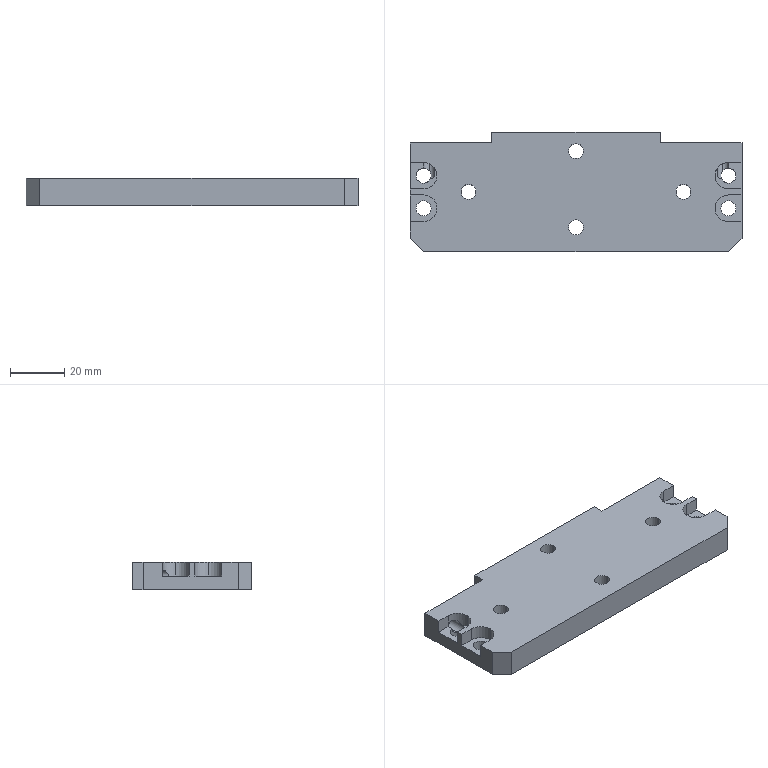Part | NX | features BREP 1 | 1 solid | 72 faces | box 122 x 44 x 10 mm | volume 46227 mm3 | cylinder 38 | plane 28 | cone 6 | commonest cylinder face diameters 5.5 x16 9.8 x14 4.2 x8